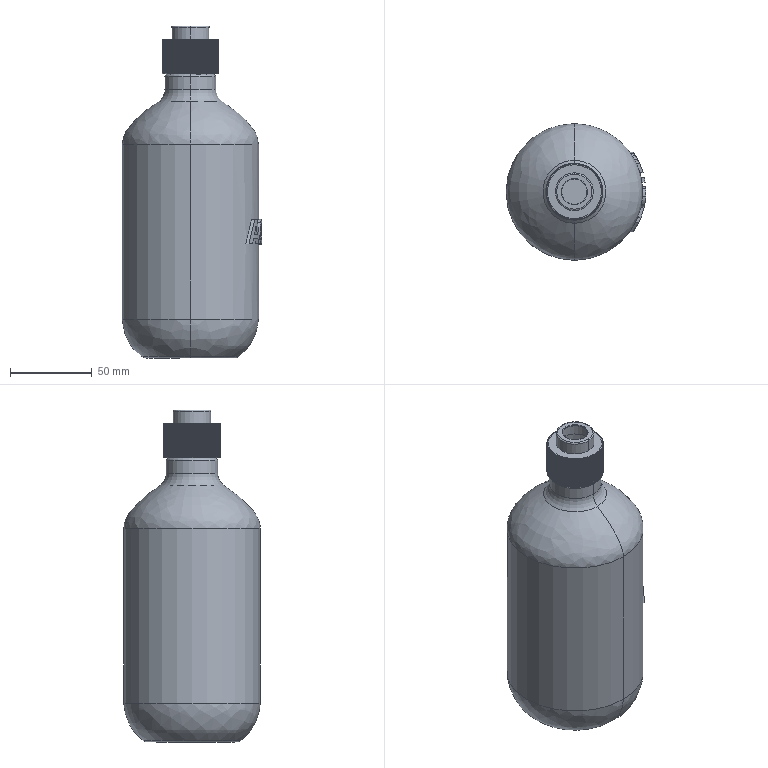Part | SolidWorks | features BaseBody 2 | 2 solids | 898 faces | box 85.56 x 83.56 x 203.378 mm | volume 49544 mm3 | cylinder 359 | spline 260 | sphere 220 | plane 31 | torus 28 | commonest cylinder face diameters 0.3 x220 0.4 x110 83.56 x9 15.567 x2 21.567 x2 23.167 x2